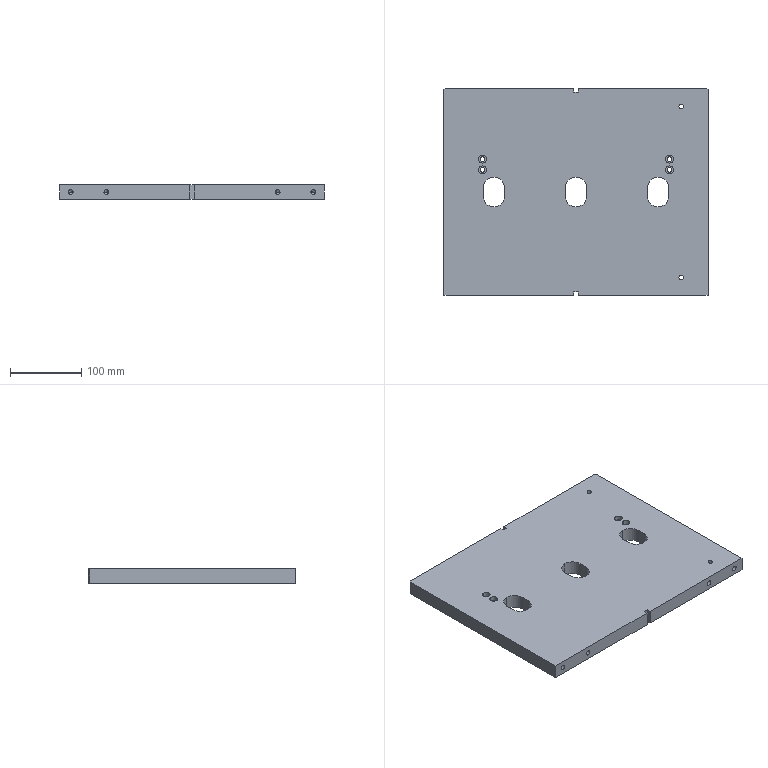CAM job | NX | 3-axis milling, drilling | part box 370 x 290 x 20 mm | stock box 374 x 294 x 21 mm
Tools:
number,name,description,diameter,corner_radius,flute_length,length,flutes
1,D63,Milling Tool-5 Parameters,63.0,0.0,50.0,75.0,2
7,D6A45,Milling Tool-5 Parameters,6.0,0.0,3.0,3.0,2
16,6.6ZT,Drilling Tool,6.6,0.0,35.0,50.0,2
10,D10,Milling Tool-5 Parameters,10.0,0.0,50.0,75.0,2
6,D6,Milling Tool-5 Parameters,6.0,0.0,50.0,75.0,2
4,D4,Milling Tool-5 Parameters,4.0,0.0,50.0,75.0,2
11,D10JING,Milling Tool-5 Parameters,10.0,0.0,50.0,75.0,2
Operations:
program,operation,operation_type,tool,method,geometry_group,spindle_rpm,surface_speed,feed_per_tooth,feed_cut,feed_plunge,cut_length_mm,path_length_mm,cut_time_min,machine_time_min
1-373-293-20毛胚AB胶,FLOOR_WALL,VolumeBased25DMillingOperation,D63,METHOD,A,6500.0,1286.0,0.0962,1250.0,100.0,4650.797,4704.797,3.721,3.726
1-373-293-20毛胚AB胶,DRILLING_COPY_1,Operation,D6A45,METHOD,A,3000.0,56.0,0.0333,200.0,0.0,30.6,682.77,0.153,0.2182
1-373-293-20毛胚AB胶,DRILLING_COPY_1_COPY_COPY_2,Operation,6.6ZT,METHOD,A,2000.0,15.0,0.0375,150.0,0.0,50.966,404.95,0.3398,0.3752
1-373-293-20毛胚AB胶,DRILLING_COPY_1_COPY_COPY_2_COPY,Operation,6.6ZT,METHOD,A,2000.0,15.0,0.0375,150.0,0.0,101.931,565.474,0.6795,0.7259
1-373-293-20毛胚AB胶,ZLEVEL_PROFILE,ZLevelMilling,D10,METHOD,A,7000.0,219.0,0.2143,3000.0,1000.0,27115.03,27191.43,9.07,9.077
1-373-293-20毛胚AB胶,ZLEVEL_PROFILE_COPY_COPY,ZLevelMilling,D10,METHOD,A,7000.0,219.0,0.2143,3000.0,1000.0,3591.63,4054.265,1.293,1.339
1-373-293-20毛胚AB胶,ZLEVEL_PROFILE_COPY,ZLevelMilling,D10,METHOD,A,7000.0,219.0,0.2143,3000.0,1000.0,5491.282,5940.365,1.926,1.971
1-373-293-20毛胚AB胶,HOLE_MILLING,CylinderMilling,D6,METHOD,A,7000.0,131.0,0.1071,1500.0,100.0,961.766,1517.795,0.6412,0.6968
1-373-293-20毛胚AB胶,ZLEVEL_PROFILE_COPY_1,ZLevelMilling,D4,METHOD,A,7000.0,87.0,0.1071,1500.0,1000.0,1432.008,2332.204,0.9888,1.079
1-373-293-20毛胚AB胶,ZLEVEL_PROFILE_COPY_COPY_1_COPY_COPY_COPY_1,ZLevelMilling,D10JING,METHOD,A,7000.0,219.0,0.0714,1000.0,100.0,232.912,777.5,0.2329,0.2874
1-373-293-20毛胚AB胶,ZLEVEL_PROFILE_COPY_1_COPY_COPY_COPY_COPY_2_COPY,ZLevelMilling,D6A45,METHOD,A,7000.0,131.0,0.0714,1000.0,1000.0,1861.36,4083.719,1.861,2.084
1-373-293-20毛胚AB胶,ZLEVEL_PROFILE_COPY_1_1,ZLevelMilling,D10JING,METHOD,A,7000.0,219.0,0.0714,1000.0,1000.0,4455.038,4532.788,4.455,4.463